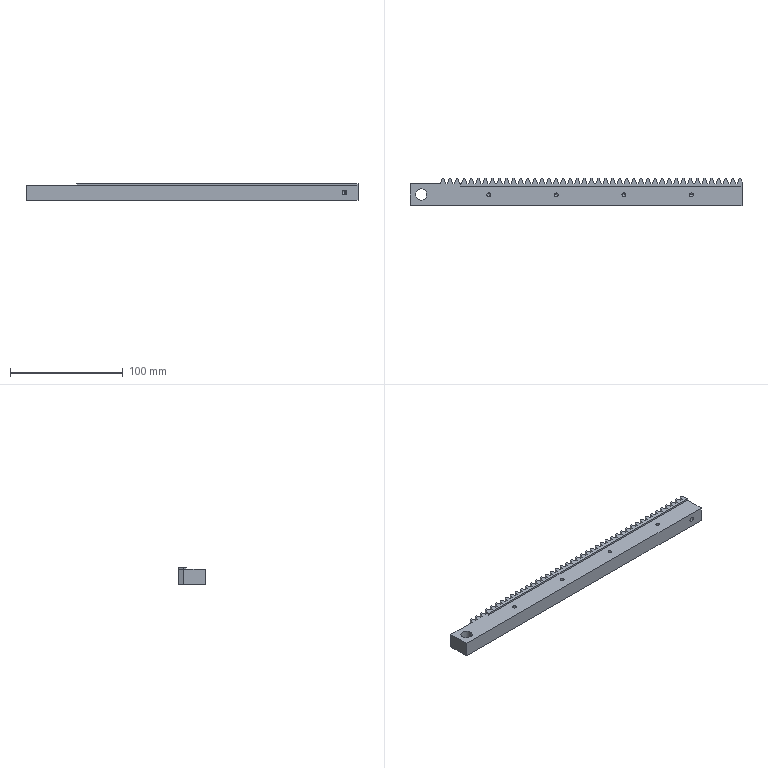Part | SolidWorks | features ICE 46, Draft 42, HoleWzd 5, Extrusion 1 | 1 solid | 215 faces | box 295 x 24 x 15 mm | volume 85099 mm3 | plane 180 | cylinder 20 | cone 15 | commonest cylinder face diameters 4.2 x10 3.3 x8 10 x2